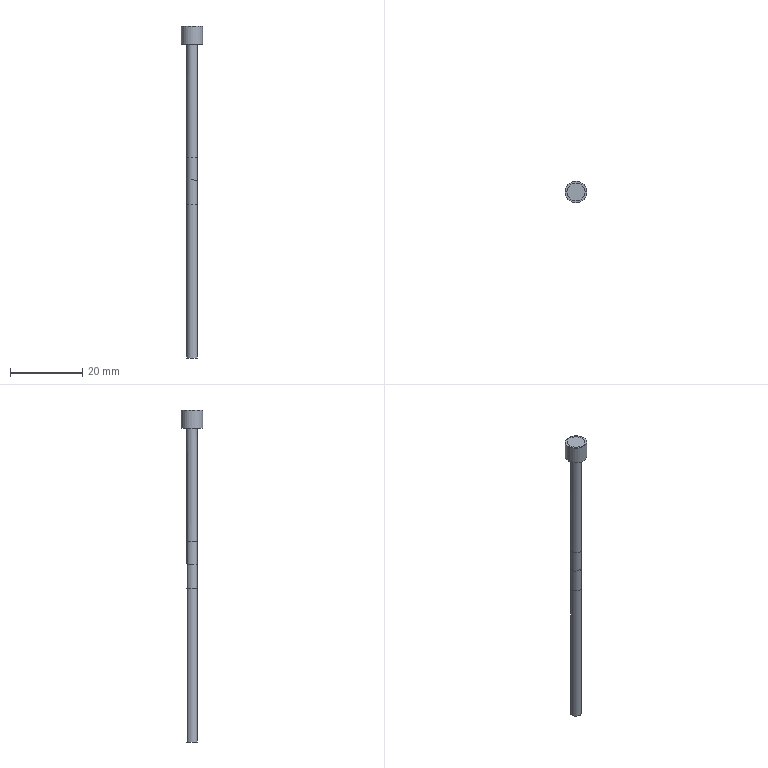Part | NX | features BREP 3 | 3 solids | 38 faces | box 6 x 6 x 92.2 mm | volume 1255 mm3 | cylinder 17 | plane 17 | torus 4 | commonest cylinder face diameters 1 x4 1.1 x4 20 x4 3 x3 5 x1 6 x1
STEP:
#1=CARTESIAN_POINT('',(3.,0.,47.));
#2=VERTEX_POINT('',#1);
#3=CARTESIAN_POINT('',(0.,0.,47.));
#4=DIRECTION('',(0.,0.,-1.));
#5=DIRECTION('',(1.,0.,0.));
#6=AXIS2_PLACEMENT_3D('',#3,#4,#5);
#7=CIRCLE('',#6,3.);
#8=EDGE_CURVE('',#2,#2,#7,.T.);
#9=ORIENTED_EDGE('',*,*,#8,.F.);
#10=EDGE_LOOP('',(#9));
#11=FACE_BOUND('',#10,.T.);
#12=CARTESIAN_POINT('',(3.,0.,52.));
#13=VERTEX_POINT('',#12);
#14=CARTESIAN_POINT('',(0.,0.,52.));
#15=DIRECTION('',(0.,0.,-1.));
#16=DIRECTION('',(1.,0.,0.));
#17=AXIS2_PLACEMENT_3D('',#14,#15,#16);
#18=CIRCLE('',#17,3.);
#19=EDGE_CURVE('',#13,#13,#18,.T.);
#20=ORIENTED_EDGE('',*,*,#19,.T.);
#21=EDGE_LOOP('',(#20));
#22=FACE_BOUND('',#21,.T.);
#23=CARTESIAN_POINT('',(0.,0.,47.));
#24=DIRECTION('',(0.,0.,1.));
#25=DIRECTION('',(-1.,0.,0.));
#26=AXIS2_PLACEMENT_3D('',#23,#24,#25);
#27=CYLINDRICAL_SURFACE('',#26,3.);
#28=ADVANCED_FACE('',(#11,#22),#27,.T.);
#29=CARTESIAN_POINT('',(-1.5,0.,47.));
#30=VERTEX_POINT('',#29);
#31=CARTESIAN_POINT('',(0.,0.,47.));
#32=DIRECTION('',(0.,0.,-1.));
#33=DIRECTION('',(-1.,0.,0.));
#34=AXIS2_PLACEMENT_3D('',#31,#32,#33);
#35=CIRCLE('',#34,1.5);
#36=EDGE_CURVE('',#30,#30,#35,.T.);
#37=ORIENTED_EDGE('',*,*,#36,.F.);
#38=EDGE_LOOP('',(#37));
#39=FACE_BOUND('',#38,.T.);
#40=ORIENTED_EDGE('',*,*,#8,.T.);
#41=EDGE_LOOP('',(#40));
#42=FACE_BOUND('',#41,.T.);
#43=CARTESIAN_POINT('',(0.,0.,47.));
#44=DIRECTION('',(0.,0.,-1.));
#45=DIRECTION('',(1.,0.,0.));
#46=AXIS2_PLACEMENT_3D('',#43,#44,#45);
#47=PLANE('',#46);
#48=ADVANCED_FACE('',(#39,#42),#47,.T.);
#49=ORIENTED_EDGE('',*,*,#19,.F.);
#50=EDGE_LOOP('',(#49));
#51=FACE_BOUND('',#50,.T.);
#52=CARTESIAN_POINT('',(0.,0.,52.));
#53=DIRECTION('',(0.,0.,-1.));
#54=DIRECTION('',(1.,0.,0.));
#55=AXIS2_PLACEMENT_3D('',#52,#53,#54);
#56=PLANE('',#55);
#57=ADVANCED_FACE('',(#51),#56,.F.);
#58=CARTESIAN_POINT('',(-0.25,0.7001,2.4));
#59=VERTEX_POINT('',#58);
#60=CARTESIAN_POINT('',(-0.8001,0.15,2.4));
#61=VERTEX_POINT('',#60);
#62=CARTESIAN_POINT('',(-0.25,0.15,2.4));
#63=DIRECTION('',(0.,0.,1.));
#64=DIRECTION('',(1.,0.,0.));
#65=AXIS2_PLACEMENT_3D('',#62,#63,#64);
#66=CIRCLE('',#65,0.5501);
#67=EDGE_CURVE('',#59,#61,#66,.T.);
#68=ORIENTED_EDGE('',*,*,#67,.T.);
#69=CARTESIAN_POINT('',(-0.8001,-0.15,2.4));
#70=VERTEX_POINT('',#69);
#71=CARTESIAN_POINT('',(-0.8001,0.15,2.4));
#72=DIRECTION('',(0.,-1.,0.));
#73=VECTOR('',#72,1000.);
#74=LINE('',#71,#73);
#75=EDGE_CURVE('',#61,#70,#74,.T.);
#76=ORIENTED_EDGE('',*,*,#75,.T.);
#77=CARTESIAN_POINT('',(-0.25,-0.7001,2.4));
#78=VERTEX_POINT('',#77);
#79=CARTESIAN_POINT('',(-0.25,-0.15,2.4));
#80=DIRECTION('',(0.,0.,1.));
#81=DIRECTION('',(1.,0.,0.));
#82=AXIS2_PLACEMENT_3D('',#79,#80,#81);
#83=CIRCLE('',#82,0.5501);
#84=EDGE_CURVE('',#70,#78,#83,.T.);
#85=ORIENTED_EDGE('',*,*,#84,.T.);
#86=CARTESIAN_POINT('',(0.25,-0.7001,2.4));
#87=VERTEX_POINT('',#86);
#88=CARTESIAN_POINT('',(-0.25,-0.7001,2.4));
#89=DIRECTION('',(1.,0.,0.));
#90=VECTOR('',#89,1000.);
#91=LINE('',#88,#90);
#92=EDGE_CURVE('',#78,#87,#91,.T.);
#93=ORIENTED_EDGE('',*,*,#92,.T.);
#94=CARTESIAN_POINT('',(0.8001,-0.15,2.4));
#95=VERTEX_POINT('',#94);
#96=CARTESIAN_POINT('',(0.25,-0.15,2.4));
#97=DIRECTION('',(0.,0.,1.));
#98=DIRECTION('',(1.,0.,0.));
#99=AXIS2_PLACEMENT_3D('',#96,#97,#98);
#100=CIRCLE('',#99,0.5501);
#101=EDGE_CURVE('',#87,#95,#100,.T.);
#102=ORIENTED_EDGE('',*,*,#101,.T.);
#103=CARTESIAN_POINT('',(0.8001,0.15,2.4));
#104=VERTEX_POINT('',#103);
#105=CARTESIAN_POINT('',(0.8001,-0.15,2.4));
#106=DIRECTION('',(0.,1.,0.));
#107=VECTOR('',#106,1000.);
#108=LINE('',#105,#107);
#109=EDGE_CURVE('',#95,#104,#108,.T.);
#110=ORIENTED_EDGE('',*,*,#109,.T.);
#111=CARTESIAN_POINT('',(0.25,0.7001,2.4));
#112=VERTEX_POINT('',#111);
#113=CARTESIAN_POINT('',(0.25,0.15,2.4));
#114=DIRECTION('',(0.,0.,1.));
#115=DIRECTION('',(1.,0.,0.));
#116=AXIS2_PLACEMENT_3D('',#113,#114,#115);
#117=CIRCLE('',#116,0.5501);
#118=EDGE_CURVE('',#104,#112,#117,.T.);
#119=ORIENTED_EDGE('',*,*,#118,.T.);
#120=CARTESIAN_POINT('',(0.25,0.7001,2.4));
#121=DIRECTION('',(-1.,0.,0.));
#122=VECTOR('',#121,1000.);
#123=LINE('',#120,#122);
#124=EDGE_CURVE('',#112,#59,#123,.T.);
#125=ORIENTED_EDGE('',*,*,#124,.T.);
#126=EDGE_LOOP('',(#68,#76,#85,#93,#102,#110,#119,#125));
#127=FACE_BOUND('',#126,.T.);
#128=CARTESIAN_POINT('',(-1.5,0.,2.4));
#129=VERTEX_POINT('',#128);
#130=CARTESIAN_POINT('',(0.,0.,2.4));
#131=DIRECTION('',(0.,0.,-1.));
#132=DIRECTION('',(-1.,0.,0.));
#133=AXIS2_PLACEMENT_3D('',#130,#131,#132);
#134=CIRCLE('',#133,1.5);
#135=EDGE_CURVE('',#129,#129,#134,.T.);
#136=ORIENTED_EDGE('',*,*,#135,.T.);
#137=EDGE_LOOP('',(#136));
#138=FACE_BOUND('',#137,.T.);
#139=CARTESIAN_POINT('',(0.,0.,2.4));
#140=DIRECTION('',(0.,0.,-1.));
#141=DIRECTION('',(1.,0.,0.));
#142=AXIS2_PLACEMENT_3D('',#139,#140,#141);
#143=PLANE('',#142);
#144=ADVANCED_FACE('',(#127,#138),#143,.T.);
#145=ORIENTED_EDGE('',*,*,#135,.F.);
#146=EDGE_LOOP('',(#145));
#147=FACE_BOUND('',#146,.T.);
#148=ORIENTED_EDGE('',*,*,#36,.T.);
#149=EDGE_LOOP('',(#148));
#150=FACE_BOUND('',#149,.T.);
#151=CARTESIAN_POINT('',(0.,0.,47.));
#152=DIRECTION('',(0.,0.,-1.));
#153=DIRECTION('',(1.,0.,0.));
#154=AXIS2_PLACEMENT_3D('',#151,#152,#153);
#155=CYLINDRICAL_SURFACE('',#154,1.5);
#156=ADVANCED_FACE('',(#147,#150),#155,.T.);
#157=CARTESIAN_POINT('',(-0.25,-0.7001,-3.6));
#158=VERTEX_POINT('',#157);
#159=CARTESIAN_POINT('',(-0.25,-0.7001,0.));
#160=DIRECTION('',(0.,0.,-1.));
#161=VECTOR('',#160,1000.);
#162=LINE('',#159,#161);
#163=EDGE_CURVE('',#78,#158,#162,.T.);
#164=ORIENTED_EDGE('',*,*,#163,.T.);
#165=CARTESIAN_POINT('',(0.25,-0.7001,-3.6));
#166=VERTEX_POINT('',#165);
#167=CARTESIAN_POINT('',(-0.25,-0.7001,-3.6));
#168=DIRECTION('',(1.,0.,0.));
#169=VECTOR('',#168,1000.);
#170=LINE('',#167,#169);
#171=EDGE_CURVE('',#158,#166,#170,.T.);
#172=ORIENTED_EDGE('',*,*,#171,.T.);
#173=CARTESIAN_POINT('',(0.25,-0.7001,0.));
#174=DIRECTION('',(0.,0.,-1.));
#175=VECTOR('',#174,1000.);
#176=LINE('',#173,#175);
#177=EDGE_CURVE('',#87,#166,#176,.T.);
#178=ORIENTED_EDGE('',*,*,#177,.F.);
#179=ORIENTED_EDGE('',*,*,#92,.F.);
#180=EDGE_LOOP('',(#164,#172,#178,#179));
#181=FACE_BOUND('',#180,.T.);
#182=CARTESIAN_POINT('',(-0.25,-0.7001,0.));
#183=DIRECTION('',(0.,-1.,0.));
#184=DIRECTION('',(-1.,0.,0.));
#185=AXIS2_PLACEMENT_3D('',#182,#183,#184);
#186=PLANE('',#185);
#187=ADVANCED_FACE('',(#181),#186,.T.);
#188=ORIENTED_EDGE('',*,*,#177,.T.);
#189=CARTESIAN_POINT('',(0.8001,-0.15,-3.6));
#190=VERTEX_POINT('',#189);
#191=CARTESIAN_POINT('',(0.25,-0.15,-3.6));
#192=DIRECTION('',(0.,0.,1.));
#193=DIRECTION('',(1.,0.,0.));
#194=AXIS2_PLACEMENT_3D('',#191,#192,#193);
#195=CIRCLE('',#194,0.5501);
#196=EDGE_CURVE('',#166,#190,#195,.T.);
#197=ORIENTED_EDGE('',*,*,#196,.T.);
#198=CARTESIAN_POINT('',(0.8001,-0.15,0.));
#199=DIRECTION('',(0.,0.,-1.));
#200=VECTOR('',#199,1000.);
#201=LINE('',#198,#200);
#202=EDGE_CURVE('',#95,#190,#201,.T.);
#203=ORIENTED_EDGE('',*,*,#202,.F.);
#204=ORIENTED_EDGE('',*,*,#101,.F.);
#205=EDGE_LOOP('',(#188,#197,#203,#204));
#206=FACE_BOUND('',#205,.T.);
#207=CARTESIAN_POINT('',(0.25,-0.15,0.));
#208=DIRECTION('',(0.,0.,1.));
#209=DIRECTION('',(-1.,0.,0.));
#210=AXIS2_PLACEMENT_3D('',#207,#208,#209);
#211=CYLINDRICAL_SURFACE('',#210,0.5501);
#212=ADVANCED_FACE('',(#206),#211,.T.);
#213=ORIENTED_EDGE('',*,*,#202,.T.);
#214=CARTESIAN_POINT('',(0.8001,0.15,-3.6));
#215=VERTEX_POINT('',#214);
#216=CARTESIAN_POINT('',(0.8001,-0.15,-3.6));
#217=DIRECTION('',(0.,1.,0.));
#218=VECTOR('',#217,1000.);
#219=LINE('',#216,#218);
#220=EDGE_CURVE('',#190,#215,#219,.T.);
#221=ORIENTED_EDGE('',*,*,#220,.T.);
#222=CARTESIAN_POINT('',(0.8001,0.15,0.));
#223=DIRECTION('',(0.,0.,-1.));
#224=VECTOR('',#223,1000.);
#225=LINE('',#222,#224);
#226=EDGE_CURVE('',#104,#215,#225,.T.);
#227=ORIENTED_EDGE('',*,*,#226,.F.);
#228=ORIENTED_EDGE('',*,*,#109,.F.);
#229=EDGE_LOOP('',(#213,#221,#227,#228));
#230=FACE_BOUND('',#229,.T.);
#231=CARTESIAN_POINT('',(0.8001,-0.15,0.));
#232=DIRECTION('',(1.,0.,0.));
#233=DIRECTION('',(0.,-1.,0.));
#234=AXIS2_PLACEMENT_3D('',#231,#232,#233);
#235=PLANE('',#234);
#236=ADVANCED_FACE('',(#230),#235,.T.);
#237=ORIENTED_EDGE('',*,*,#226,.T.);
#238=CARTESIAN_POINT('',(0.25,0.7001,-3.6));
#239=VERTEX_POINT('',#238);
#240=CARTESIAN_POINT('',(0.25,0.15,-3.6));
#241=DIRECTION('',(0.,0.,1.));
#242=DIRECTION('',(1.,0.,0.));
#243=AXIS2_PLACEMENT_3D('',#240,#241,#242);
#244=CIRCLE('',#243,0.5501);
#245=EDGE_CURVE('',#215,#239,#244,.T.);
#246=ORIENTED_EDGE('',*,*,#245,.T.);
#247=CARTESIAN_POINT('',(0.25,0.7001,0.));
#248=DIRECTION('',(0.,0.,-1.));
#249=VECTOR('',#248,1000.);
#250=LINE('',#247,#249);
#251=EDGE_CURVE('',#112,#239,#250,.T.);
#252=ORIENTED_EDGE('',*,*,#251,.F.);
#253=ORIENTED_EDGE('',*,*,#118,.F.);
#254=EDGE_LOOP('',(#237,#246,#252,#253));
#255=FACE_BOUND('',#254,.T.);
#256=CARTESIAN_POINT('',(0.25,0.15,0.));
#257=DIRECTION('',(0.,0.,1.));
#258=DIRECTION('',(-1.,0.,0.));
#259=AXIS2_PLACEMENT_3D('',#256,#257,#258);
#260=CYLINDRICAL_SURFACE('',#259,0.5501);
#261=ADVANCED_FACE('',(#255),#260,.T.);
#262=ORIENTED_EDGE('',*,*,#251,.T.);
#263=CARTESIAN_POINT('',(-0.25,0.7001,-3.6));
#264=VERTEX_POINT('',#263);
#265=CARTESIAN_POINT('',(0.25,0.7001,-3.6));
#266=DIRECTION('',(-1.,0.,0.));
#267=VECTOR('',#266,1000.);
#268=LINE('',#265,#267);
#269=EDGE_CURVE('',#239,#264,#268,.T.);
#270=ORIENTED_EDGE('',*,*,#269,.T.);
#271=CARTESIAN_POINT('',(-0.25,0.7001,0.));
#272=DIRECTION('',(0.,0.,-1.));
#273=VECTOR('',#272,1000.);
#274=LINE('',#271,#273);
#275=EDGE_CURVE('',#59,#264,#274,.T.);
#276=ORIENTED_EDGE('',*,*,#275,.F.);
#277=ORIENTED_EDGE('',*,*,#124,.F.);
#278=EDGE_LOOP('',(#262,#270,#276,#277));
#279=FACE_BOUND('',#278,.T.);
#280=CARTESIAN_POINT('',(0.25,0.7001,0.));
#281=DIRECTION('',(0.,1.,0.));
#282=DIRECTION('',(1.,0.,0.));
#283=AXIS2_PLACEMENT_3D('',#280,#281,#282);
#284=PLANE('',#283);
#285=ADVANCED_FACE('',(#279),#284,.T.);
#286=ORIENTED_EDGE('',*,*,#275,.T.);
#287=CARTESIAN_POINT('',(-0.8001,0.15,-3.6));
#288=VERTEX_POINT('',#287);
#289=CARTESIAN_POINT('',(-0.25,0.15,-3.6));
#290=DIRECTION('',(0.,0.,1.));
#291=DIRECTION('',(1.,0.,0.));
#292=AXIS2_PLACEMENT_3D('',#289,#290,#291);
#293=CIRCLE('',#292,0.5501);
#294=EDGE_CURVE('',#264,#288,#293,.T.);
#295=ORIENTED_EDGE('',*,*,#294,.T.);
#296=CARTESIAN_POINT('',(-0.8001,0.15,0.));
#297=DIRECTION('',(0.,0.,-1.));
#298=VECTOR('',#297,1000.);
#299=LINE('',#296,#298);
#300=EDGE_CURVE('',#61,#288,#299,.T.);
#301=ORIENTED_EDGE('',*,*,#300,.F.);
#302=ORIENTED_EDGE('',*,*,#67,.F.);
#303=EDGE_LOOP('',(#286,#295,#301,#302));
#304=FACE_BOUND('',#303,.T.);
#305=CARTESIAN_POINT('',(-0.25,0.15,0.));
#306=DIRECTION('',(0.,0.,1.));
#307=DIRECTION('',(-1.,0.,0.));
#308=AXIS2_PLACEMENT_3D('',#305,#306,#307);
#309=CYLINDRICAL_SURFACE('',#308,0.5501);
#310=ADVANCED_FACE('',(#304),#309,.T.);
#311=ORIENTED_EDGE('',*,*,#300,.T.);
#312=CARTESIAN_POINT('',(-0.8001,-0.15,-3.6));
#313=VERTEX_POINT('',#312);
#314=CARTESIAN_POINT('',(-0.8001,0.15,-3.6));
#315=DIRECTION('',(0.,-1.,0.));
#316=VECTOR('',#315,1000.);
#317=LINE('',#314,#316);
#318=EDGE_CURVE('',#288,#313,#317,.T.);
#319=ORIENTED_EDGE('',*,*,#318,.T.);
#320=CARTESIAN_POINT('',(-0.8001,-0.15,0.));
#321=DIRECTION('',(0.,0.,-1.));
#322=VECTOR('',#321,1000.);
#323=LINE('',#320,#322);
#324=EDGE_CURVE('',#70,#313,#323,.T.);
#325=ORIENTED_EDGE('',*,*,#324,.F.);
#326=ORIENTED_EDGE('',*,*,#75,.F.);
#327=EDGE_LOOP('',(#311,#319,#325,#326));
#328=FACE_BOUND('',#327,.T.);
#329=CARTESIAN_POINT('',(-0.8001,0.15,0.));
#330=DIRECTION('',(-1.,0.,0.));
#331=DIRECTION('',(0.,1.,0.));
#332=AXIS2_PLACEMENT_3D('',#329,#330,#331);
#333=PLANE('',#332);
#334=ADVANCED_FACE('',(#328),#333,.T.);
#335=ORIENTED_EDGE('',*,*,#84,.F.);
#336=ORIENTED_EDGE('',*,*,#324,.T.);
#337=CARTESIAN_POINT('',(-0.25,-0.15,-3.6));
#338=DIRECTION('',(0.,0.,1.));
#339=DIRECTION('',(1.,0.,0.));
#340=AXIS2_PLACEMENT_3D('',#337,#338,#339);
#341=CIRCLE('',#340,0.5501);
#342=EDGE_CURVE('',#313,#158,#341,.T.);
#343=ORIENTED_EDGE('',*,*,#342,.T.);
#344=ORIENTED_EDGE('',*,*,#163,.F.);
#345=EDGE_LOOP('',(#335,#336,#343,#344));
#346=FACE_BOUND('',#345,.T.);
#347=CARTESIAN_POINT('',(-0.25,-0.15,0.));
#348=DIRECTION('',(0.,0.,1.));
#349=DIRECTION('',(-1.,0.,0.));
#350=AXIS2_PLACEMENT_3D('',#347,#348,#349);
#351=CYLINDRICAL_SURFACE('',#350,0.5501);
#352=ADVANCED_FACE('',(#346),#351,.T.);
#353=ORIENTED_EDGE('',*,*,#318,.F.);
#354=ORIENTED_EDGE('',*,*,#294,.F.);
#355=ORIENTED_EDGE('',*,*,#269,.F.);
#356=ORIENTED_EDGE('',*,*,#245,.F.);
#357=ORIENTED_EDGE('',*,*,#220,.F.);
#358=ORIENTED_EDGE('',*,*,#196,.F.);
#359=ORIENTED_EDGE('',*,*,#171,.F.);
#360=ORIENTED_EDGE('',*,*,#342,.F.);
#361=EDGE_LOOP('',(#353,#354,#355,#356,#357,#358,#359,#360));
#362=FACE_BOUND('',#361,.T.);
#363=CARTESIAN_POINT('',(8.223,0.1277,-3.6));
#364=DIRECTION('',(0.,0.,1.));
#365=DIRECTION('',(-1.,0.,0.));
#366=AXIS2_PLACEMENT_3D('',#363,#364,#365);
#367=PLANE('',#366);
#368=ADVANCED_FACE('',(#362),#367,.F.);
#369=CLOSED_SHELL('',(#28,#48,#57,#144,#156,#187,#212,#236,#261,#285,#310,#334,#352,#368));
#370=MANIFOLD_SOLID_BREP('',#369);
#371=CARTESIAN_POINT('',(2.5,0.,47.));
#372=VERTEX_POINT('',#371);
#373=CARTESIAN_POINT('',(0.,0.,47.));
#374=DIRECTION('',(0.,0.,-1.));
#375=DIRECTION('',(1.,0.,0.));
#376=AXIS2_PLACEMENT_3D('',#373,#374,#375);
#377=CIRCLE('',#376,2.5);
#378=EDGE_CURVE('',#372,#372,#377,.T.);
#379=ORIENTED_EDGE('',*,*,#378,.F.);
#380=EDGE_LOOP('',(#379));
#381=FACE_BOUND('',#380,.T.);
#382=CARTESIAN_POINT('',(2.5,0.,52.));
#383=VERTEX_POINT('',#382);
#384=CARTESIAN_POINT('',(0.,0.,52.));
#385=DIRECTION('',(0.,0.,-1.));
#386=DIRECTION('',(1.,0.,0.));
#387=AXIS2_PLACEMENT_3D('',#384,#385,#386);
#388=CIRCLE('',#387,2.5);
#389=EDGE_CURVE('',#383,#383,#388,.T.);
#390=ORIENTED_EDGE('',*,*,#389,.T.);
#391=EDGE_LOOP('',(#390));
#392=FACE_BOUND('',#391,.T.);
#393=CARTESIAN_POINT('',(0.,0.,47.));
#394=DIRECTION('',(0.,0.,1.));
#395=DIRECTION('',(-1.,0.,0.));
#396=AXIS2_PLACEMENT_3D('',#393,#394,#395);
#397=CYLINDRICAL_SURFACE('',#396,2.5);
#398=ADVANCED_FACE('',(#381,#392),#397,.T.);
#399=CARTESIAN_POINT('',(-1.5,0.,47.));
#400=VERTEX_POINT('',#399);
#401=CARTESIAN_POINT('',(0.,0.,47.));
#402=DIRECTION('',(0.,0.,-1.));
#403=DIRECTION('',(-1.,0.,0.));
#404=AXIS2_PLACEMENT_3D('',#401,#402,#403);
#405=CIRCLE('',#404,1.5);
#406=EDGE_CURVE('',#400,#400,#405,.T.);
#407=ORIENTED_EDGE('',*,*,#406,.F.);
#408=EDGE_LOOP('',(#407));
#409=FACE_BOUND('',#408,.T.);
#410=ORIENTED_EDGE('',*,*,#378,.T.);
#411=EDGE_LOOP('',(#410));
#412=FACE_BOUND('',#411,.T.);
#413=CARTESIAN_POINT('',(0.,0.,47.));
#414=DIRECTION('',(0.,0.,-1.));
#415=DIRECTION('',(1.,0.,0.));
#416=AXIS2_PLACEMENT_3D('',#413,#414,#415);
#417=PLANE('',#416);
#418=ADVANCED_FACE('',(#409,#412),#417,.T.);
#419=ORIENTED_EDGE('',*,*,#389,.F.);
#420=EDGE_LOOP('',(#419));
#421=FACE_BOUND('',#420,.T.);
#422=CARTESIAN_POINT('',(0.,0.,52.));
#423=DIRECTION('',(0.,0.,-1.));
#424=DIRECTION('',(1.,0.,0.));
#425=AXIS2_PLACEMENT_3D('',#422,#423,#424);
#426=PLANE('',#425);
#427=ADVANCED_FACE('',(#421),#426,.F.);
#428=ORIENTED_EDGE('',*,*,#406,.T.);
#429=EDGE_LOOP('',(#428));
#430=FACE_BOUND('',#429,.T.);
#431=CARTESIAN_POINT('',(-1.492,-0.15,9.181));
#432=VERTEX_POINT('',#431);
#433=CARTESIAN_POINT('',(-1.492,0.15,9.181));
#434=VERTEX_POINT('',#433);
#435=CARTESIAN_POINT('',(-1.492,-0.15,9.181));
#436=CARTESIAN_POINT('',(-1.502,-0.05157,9.205));
#437=CARTESIAN_POINT('',(-1.502,0.05153,9.205));
#438=CARTESIAN_POINT('',(-1.492,0.15,9.181));
#439=B_SPLINE_CURVE_WITH_KNOTS('',3,(#435,#436,#437,#438),.UNSPECIFIED.,.F.,.F.,(4,4),(0.,0.0003013),.UNSPECIFIED.);
#440=EDGE_CURVE('',#432,#434,#439,.T.);
#441=ORIENTED_EDGE('',*,*,#440,.F.);
#442=CARTESIAN_POINT('',(-0.25,-1.479,9.386));
#443=VERTEX_POINT('',#442);
#444=CARTESIAN_POINT('',(-0.25,-1.479,9.386));
#445=CARTESIAN_POINT('',(-0.8693,-1.374,9.146));
#446=CARTESIAN_POINT('',(-1.427,-0.8014,9.021));
#447=CARTESIAN_POINT('',(-1.492,-0.15,9.181));
#448=B_SPLINE_CURVE_WITH_KNOTS('',3,(#444,#445,#446,#447),.UNSPECIFIED.,.F.,.F.,(4,4),(0.,0.001996),.UNSPECIFIED.);
#449=EDGE_CURVE('',#443,#432,#448,.T.);
#450=ORIENTED_EDGE('',*,*,#449,.F.);
#451=CARTESIAN_POINT('',(0.25,-1.479,9.386));
#452=VERTEX_POINT('',#451);
#453=CARTESIAN_POINT('',(0.25,-1.479,9.386));
#454=CARTESIAN_POINT('',(0.09098,-1.506,9.448));
#455=CARTESIAN_POINT('',(-0.09088,-1.506,9.448));
#456=CARTESIAN_POINT('',(-0.25,-1.479,9.386));
#457=B_SPLINE_CURVE_WITH_KNOTS('',3,(#453,#454,#455,#456),.UNSPECIFIED.,.F.,.F.,(4,4),(0.,0.0005114),.UNSPECIFIED.);
#458=EDGE_CURVE('',#452,#443,#457,.T.);
#459=ORIENTED_EDGE('',*,*,#458,.F.);
#460=CARTESIAN_POINT('',(1.492,-0.15,9.181));
#461=VERTEX_POINT('',#460);
#462=CARTESIAN_POINT('',(1.492,-0.15,9.181));
#463=CARTESIAN_POINT('',(1.427,-0.8,9.021));
#464=CARTESIAN_POINT('',(0.8687,-1.374,9.146));
#465=CARTESIAN_POINT('',(0.25,-1.479,9.386));
#466=B_SPLINE_CURVE_WITH_KNOTS('',3,(#462,#463,#464,#465),.UNSPECIFIED.,.F.,.F.,(4,4),(0.,0.00199),.UNSPECIFIED.);
#467=EDGE_CURVE('',#461,#452,#466,.T.);
#468=ORIENTED_EDGE('',*,*,#467,.F.);
#469=CARTESIAN_POINT('',(1.492,0.15,9.181));
#470=VERTEX_POINT('',#469);
#471=CARTESIAN_POINT('',(1.492,0.15,9.181));
#472=CARTESIAN_POINT('',(1.502,0.05157,9.205));
#473=CARTESIAN_POINT('',(1.502,-0.05153,9.205));
#474=CARTESIAN_POINT('',(1.492,-0.15,9.181));
#475=B_SPLINE_CURVE_WITH_KNOTS('',3,(#471,#472,#473,#474),.UNSPECIFIED.,.F.,.F.,(4,4),(0.,0.0003013),.UNSPECIFIED.);
#476=EDGE_CURVE('',#470,#461,#475,.T.);
#477=ORIENTED_EDGE('',*,*,#476,.F.);
#478=CARTESIAN_POINT('',(0.25,1.479,9.386));
#479=VERTEX_POINT('',#478);
#480=CARTESIAN_POINT('',(0.25,1.479,9.386));
#481=CARTESIAN_POINT('',(0.8693,1.374,9.146));
#482=CARTESIAN_POINT('',(1.427,0.8014,9.021));
#483=CARTESIAN_POINT('',(1.492,0.15,9.181));
#484=B_SPLINE_CURVE_WITH_KNOTS('',3,(#480,#481,#482,#483),.UNSPECIFIED.,.F.,.F.,(4,4),(0.,0.001996),.UNSPECIFIED.);
#485=EDGE_CURVE('',#479,#470,#484,.T.);
#486=ORIENTED_EDGE('',*,*,#485,.F.);
#487=CARTESIAN_POINT('',(-0.25,1.479,9.386));
#488=VERTEX_POINT('',#487);
#489=CARTESIAN_POINT('',(-0.25,1.479,9.386));
#490=CARTESIAN_POINT('',(-0.09098,1.506,9.448));
#491=CARTESIAN_POINT('',(0.09088,1.506,9.448));
#492=CARTESIAN_POINT('',(0.25,1.479,9.386));
#493=B_SPLINE_CURVE_WITH_KNOTS('',3,(#489,#490,#491,#492),.UNSPECIFIED.,.F.,.F.,(4,4),(0.,0.0005114),.UNSPECIFIED.);
#494=EDGE_CURVE('',#488,#479,#493,.T.);
#495=ORIENTED_EDGE('',*,*,#494,.F.);
#496=CARTESIAN_POINT('',(-1.492,0.15,9.181));
#497=CARTESIAN_POINT('',(-1.427,0.8,9.021));
#498=CARTESIAN_POINT('',(-0.8687,1.374,9.146));
#499=CARTESIAN_POINT('',(-0.25,1.479,9.386));
#500=B_SPLINE_CURVE_WITH_KNOTS('',3,(#496,#497,#498,#499),.UNSPECIFIED.,.F.,.F.,(4,4),(0.,0.00199),.UNSPECIFIED.);
#501=EDGE_CURVE('',#434,#488,#500,.T.);
#502=ORIENTED_EDGE('',*,*,#501,.F.);
#503=EDGE_LOOP('',(#441,#450,#459,#468,#477,#486,#495,#502));
#504=FACE_BOUND('',#503,.T.);
#505=CARTESIAN_POINT('',(0.,0.,47.));
#506=DIRECTION('',(0.,0.,-1.));
#507=DIRECTION('',(1.,0.,0.));
#508=AXIS2_PLACEMENT_3D('',#505,#506,#507);
#509=CYLINDRICAL_SURFACE('',#508,1.5);
#510=ADVANCED_FACE('',(#430,#504),#509,.T.);
#511=CARTESIAN_POINT('',(-0.7501,-0.15,5.4));
#512=VERTEX_POINT('',#511);
#513=CARTESIAN_POINT('',(-10.75,-0.15,5.4));
#514=DIRECTION('',(0.,-1.,0.));
#515=DIRECTION('',(1.,0.,0.));
#516=AXIS2_PLACEMENT_3D('',#513,#514,#515);
#517=CIRCLE('',#516,10.);
#518=EDGE_CURVE('',#512,#432,#517,.T.);
#519=ORIENTED_EDGE('',*,*,#518,.T.);
#520=ORIENTED_EDGE('',*,*,#440,.T.);
#521=CARTESIAN_POINT('',(-0.7501,0.15,5.4));
#522=VERTEX_POINT('',#521);
#523=CARTESIAN_POINT('',(-10.75,0.15,5.4));
#524=DIRECTION('',(0.,-1.,0.));
#525=DIRECTION('',(0.,0.,-1.));
#526=AXIS2_PLACEMENT_3D('',#523,#524,#525);
#527=CIRCLE('',#526,10.);
#528=EDGE_CURVE('',#522,#434,#527,.T.);
#529=ORIENTED_EDGE('',*,*,#528,.F.);
#530=CARTESIAN_POINT('',(-0.7501,0.15,5.4));
#531=DIRECTION('',(0.,1.,0.));
#532=VECTOR('',#531,1000.);
#533=LINE('',#530,#532);
#534=EDGE_CURVE('',#512,#522,#533,.T.);
#535=ORIENTED_EDGE('',*,*,#534,.F.);
#536=EDGE_LOOP('',(#519,#520,#529,#535));
#537=FACE_BOUND('',#536,.T.);
#538=CARTESIAN_POINT('',(-10.75,0.15,5.4));
#539=DIRECTION('',(0.,-1.,0.));
#540=DIRECTION('',(0.,0.,1.));
#541=AXIS2_PLACEMENT_3D('',#538,#539,#540);
#542=CYLINDRICAL_SURFACE('',#541,10.);
#543=ADVANCED_FACE('',(#537),#542,.F.);
#544=CARTESIAN_POINT('',(-0.25,-0.6501,5.4));
#545=VERTEX_POINT('',#544);
#546=CARTESIAN_POINT('',(-0.25,-10.65,5.4));
#547=DIRECTION('',(1.,0.,0.));
#548=DIRECTION('',(0.,1.,0.));
#549=AXIS2_PLACEMENT_3D('',#546,#547,#548);
#550=CIRCLE('',#549,10.);
#551=EDGE_CURVE('',#545,#443,#550,.T.);
#552=ORIENTED_EDGE('',*,*,#551,.T.);
#553=ORIENTED_EDGE('',*,*,#449,.T.);
#554=ORIENTED_EDGE('',*,*,#518,.F.);
#555=CARTESIAN_POINT('',(-0.25,-0.15,5.4));
#556=DIRECTION('',(0.,0.,-1.));
#557=DIRECTION('',(-1.,0.,0.));
#558=AXIS2_PLACEMENT_3D('',#555,#556,#557);
#559=CIRCLE('',#558,0.5001);
#560=EDGE_CURVE('',#545,#512,#559,.T.);
#561=ORIENTED_EDGE('',*,*,#560,.F.);
#562=EDGE_LOOP('',(#552,#553,#554,#561));
#563=FACE_BOUND('',#562,.T.);
#564=CARTESIAN_POINT('',(-0.25,-0.15,5.4));
#565=DIRECTION('',(0.,0.,-1.));
#566=DIRECTION('',(1.,0.,0.));
#567=AXIS2_PLACEMENT_3D('',#564,#565,#566);
#568=TOROIDAL_SURFACE('',#567,10.5,10.);
#569=ADVANCED_FACE('',(#563),#568,.F.);
#570=CARTESIAN_POINT('',(0.25,-0.6501,5.4));
#571=VERTEX_POINT('',#570);
#572=CARTESIAN_POINT('',(0.25,-10.65,5.4));
#573=DIRECTION('',(1.,0.,0.));
#574=DIRECTION('',(0.,1.,0.));
#575=AXIS2_PLACEMENT_3D('',#572,#573,#574);
#576=CIRCLE('',#575,10.);
#577=EDGE_CURVE('',#571,#452,#576,.T.);
#578=ORIENTED_EDGE('',*,*,#577,.T.);
#579=ORIENTED_EDGE('',*,*,#458,.T.);
#580=ORIENTED_EDGE('',*,*,#551,.F.);
#581=CARTESIAN_POINT('',(-0.25,-0.6501,5.4));
#582=DIRECTION('',(-1.,0.,0.));
#583=VECTOR('',#582,1000.);
#584=LINE('',#581,#583);
#585=EDGE_CURVE('',#571,#545,#584,.T.);
#586=ORIENTED_EDGE('',*,*,#585,.F.);
#587=EDGE_LOOP('',(#578,#579,#580,#586));
#588=FACE_BOUND('',#587,.T.);
#589=CARTESIAN_POINT('',(-0.25,-10.65,5.4));
#590=DIRECTION('',(1.,0.,0.));
#591=DIRECTION('',(0.,-1.,0.));
#592=AXIS2_PLACEMENT_3D('',#589,#590,#591);
#593=CYLINDRICAL_SURFACE('',#592,10.);
#594=ADVANCED_FACE('',(#588),#593,.F.);
#595=CARTESIAN_POINT('',(0.7501,-0.15,5.4));
#596=VERTEX_POINT('',#595);
#597=CARTESIAN_POINT('',(10.75,-0.15,5.4));
#598=DIRECTION('',(0.,1.,0.));
#599=DIRECTION('',(0.,0.,1.));
#600=AXIS2_PLACEMENT_3D('',#597,#598,#599);
#601=CIRCLE('',#600,10.);
#602=EDGE_CURVE('',#596,#461,#601,.T.);
#603=ORIENTED_EDGE('',*,*,#602,.T.);
#604=ORIENTED_EDGE('',*,*,#467,.T.);
#605=ORIENTED_EDGE('',*,*,#577,.F.);
#606=CARTESIAN_POINT('',(0.25,-0.15,5.4));
#607=DIRECTION('',(0.,0.,-1.));
#608=DIRECTION('',(-1.,0.,0.));
#609=AXIS2_PLACEMENT_3D('',#606,#607,#608);
#610=CIRCLE('',#609,0.5001);
#611=EDGE_CURVE('',#596,#571,#610,.T.);
#612=ORIENTED_EDGE('',*,*,#611,.F.);
#613=EDGE_LOOP('',(#603,#604,#605,#612));
#614=FACE_BOUND('',#613,.T.);
#615=CARTESIAN_POINT('',(0.25,-0.15,5.4));
#616=DIRECTION('',(0.,0.,-1.));
#617=DIRECTION('',(1.,0.,0.));
#618=AXIS2_PLACEMENT_3D('',#615,#616,#617);
#619=TOROIDAL_SURFACE('',#618,10.5,10.);
#620=ADVANCED_FACE('',(#614),#619,.F.);
#621=CARTESIAN_POINT('',(0.7501,0.15,5.4));
#622=VERTEX_POINT('',#621);
#623=CARTESIAN_POINT('',(10.75,0.15,5.4));
#624=DIRECTION('',(0.,1.,0.));
#625=DIRECTION('',(0.,0.,1.));
#626=AXIS2_PLACEMENT_3D('',#623,#624,#625);
#627=CIRCLE('',#626,10.);
#628=EDGE_CURVE('',#622,#470,#627,.T.);
#629=ORIENTED_EDGE('',*,*,#628,.T.);
#630=ORIENTED_EDGE('',*,*,#476,.T.);
#631=ORIENTED_EDGE('',*,*,#602,.F.);
#632=CARTESIAN_POINT('',(0.7501,-0.15,5.4));
#633=DIRECTION('',(0.,-1.,0.));
#634=VECTOR('',#633,1000.);
#635=LINE('',#632,#634);
#636=EDGE_CURVE('',#622,#596,#635,.T.);
#637=ORIENTED_EDGE('',*,*,#636,.F.);
#638=EDGE_LOOP('',(#629,#630,#631,#637));
#639=FACE_BOUND('',#638,.T.);
#640=CARTESIAN_POINT('',(10.75,-0.15,5.4));
#641=DIRECTION('',(0.,1.,0.));
#642=DIRECTION('',(0.,0.,-1.));
#643=AXIS2_PLACEMENT_3D('',#640,#641,#642);
#644=CYLINDRICAL_SURFACE('',#643,10.);
#645=ADVANCED_FACE('',(#639),#644,.F.);
#646=CARTESIAN_POINT('',(0.25,0.6501,5.4));
#647=VERTEX_POINT('',#646);
#648=CARTESIAN_POINT('',(0.25,10.65,5.4));
#649=DIRECTION('',(-1.,0.,0.));
#650=DIRECTION('',(0.,-1.,0.));
#651=AXIS2_PLACEMENT_3D('',#648,#649,#650);
#652=CIRCLE('',#651,10.);
#653=EDGE_CURVE('',#647,#479,#652,.T.);
#654=ORIENTED_EDGE('',*,*,#653,.T.);
#655=ORIENTED_EDGE('',*,*,#485,.T.);
#656=ORIENTED_EDGE('',*,*,#628,.F.);
#657=CARTESIAN_POINT('',(0.25,0.15,5.4));
#658=DIRECTION('',(0.,0.,-1.));
#659=DIRECTION('',(-1.,0.,0.));
#660=AXIS2_PLACEMENT_3D('',#657,#658,#659);
#661=CIRCLE('',#660,0.5001);
#662=EDGE_CURVE('',#647,#622,#661,.T.);
#663=ORIENTED_EDGE('',*,*,#662,.F.);
#664=EDGE_LOOP('',(#654,#655,#656,#663));
#665=FACE_BOUND('',#664,.T.);
#666=CARTESIAN_POINT('',(0.25,0.15,5.4));
#667=DIRECTION('',(0.,0.,-1.));
#668=DIRECTION('',(1.,0.,0.));
#669=AXIS2_PLACEMENT_3D('',#666,#667,#668);
#670=TOROIDAL_SURFACE('',#669,10.5,10.);
#671=ADVANCED_FACE('',(#665),#670,.F.);
#672=CARTESIAN_POINT('',(-0.25,0.6501,5.4));
#673=VERTEX_POINT('',#672);
#674=CARTESIAN_POINT('',(-0.25,10.65,5.4));
#675=DIRECTION('',(-1.,0.,0.));
#676=DIRECTION('',(0.,-1.,0.));
#677=AXIS2_PLACEMENT_3D('',#674,#675,#676);
#678=CIRCLE('',#677,10.);
#679=EDGE_CURVE('',#673,#488,#678,.T.);
#680=ORIENTED_EDGE('',*,*,#679,.T.);
#681=ORIENTED_EDGE('',*,*,#494,.T.);
#682=ORIENTED_EDGE('',*,*,#653,.F.);
#683=CARTESIAN_POINT('',(0.25,0.6501,5.4));
#684=DIRECTION('',(1.,0.,0.));
#685=VECTOR('',#684,1000.);
#686=LINE('',#683,#685);
#687=EDGE_CURVE('',#673,#647,#686,.T.);
#688=ORIENTED_EDGE('',*,*,#687,.F.);
#689=EDGE_LOOP('',(#680,#681,#682,#688));
#690=FACE_BOUND('',#689,.T.);
#691=CARTESIAN_POINT('',(0.25,10.65,5.4));
#692=DIRECTION('',(-1.,0.,0.));
#693=DIRECTION('',(0.,1.,0.));
#694=AXIS2_PLACEMENT_3D('',#691,#692,#693);
#695=CYLINDRICAL_SURFACE('',#694,10.);
#696=ADVANCED_FACE('',(#690),#695,.F.);
#697=ORIENTED_EDGE('',*,*,#528,.T.);
#698=ORIENTED_EDGE('',*,*,#501,.T.);
#699=ORIENTED_EDGE('',*,*,#679,.F.);
#700=CARTESIAN_POINT('',(-0.25,0.15,5.4));
#701=DIRECTION('',(0.,0.,-1.));
#702=DIRECTION('',(-1.,0.,0.));
#703=AXIS2_PLACEMENT_3D('',#700,#701,#702);
#704=CIRCLE('',#703,0.5001);
#705=EDGE_CURVE('',#522,#673,#704,.T.);
#706=ORIENTED_EDGE('',*,*,#705,.F.);
#707=EDGE_LOOP('',(#697,#698,#699,#706));
#708=FACE_BOUND('',#707,.T.);
#709=CARTESIAN_POINT('',(-0.25,0.15,5.4));
#710=DIRECTION('',(0.,0.,-1.));
#711=DIRECTION('',(1.,0.,0.));
#712=AXIS2_PLACEMENT_3D('',#709,#710,#711);
#713=TOROIDAL_SURFACE('',#712,10.5,10.);
#714=ADVANCED_FACE('',(#708),#713,.F.);
#715=CARTESIAN_POINT('',(0.25,-0.65,-3.6));
#716=VERTEX_POINT('',#715);
#717=CARTESIAN_POINT('',(0.25,-0.6501,0.));
#718=DIRECTION('',(0.,0.,-1.));
#719=VECTOR('',#718,1000.);
#720=LINE('',#717,#719);
#721=EDGE_CURVE('',#571,#716,#720,.T.);
#722=ORIENTED_EDGE('',*,*,#721,.F.);
#723=ORIENTED_EDGE('',*,*,#585,.T.);
#724=CARTESIAN_POINT('',(-0.25,-0.6501,-3.6));
#725=VERTEX_POINT('',#724);
#726=CARTESIAN_POINT('',(-0.25,-0.6501,0.));
#727=DIRECTION('',(0.,0.,-1.));
#728=VECTOR('',#727,1000.);
#729=LINE('',#726,#728);
#730=EDGE_CURVE('',#545,#725,#729,.T.);
#731=ORIENTED_EDGE('',*,*,#730,.T.);
#732=CARTESIAN_POINT('',(-0.25,-0.6501,-3.6));
#733=DIRECTION('',(1.,0.,0.));
#734=VECTOR('',#733,1000.);
#735=LINE('',#732,#734);
#736=EDGE_CURVE('',#725,#716,#735,.T.);
#737=ORIENTED_EDGE('',*,*,#736,.T.);
#738=EDGE_LOOP('',(#722,#723,#731,#737));
#739=FACE_BOUND('',#738,.T.);
#740=CARTESIAN_POINT('',(-0.25,-0.6501,0.));
#741=DIRECTION('',(0.,-1.,0.));
#742=DIRECTION('',(-1.,0.,0.));
#743=AXIS2_PLACEMENT_3D('',#740,#741,#742);
#744=PLANE('',#743);
#745=ADVANCED_FACE('',(#739),#744,.T.);
#746=CARTESIAN_POINT('',(0.75,-0.15,-3.6));
#747=VERTEX_POINT('',#746);
#748=CARTESIAN_POINT('',(0.7501,-0.15,0.));
#749=DIRECTION('',(0.,0.,-1.));
#750=VECTOR('',#749,1000.);
#751=LINE('',#748,#750);
#752=EDGE_CURVE('',#596,#747,#751,.T.);
#753=ORIENTED_EDGE('',*,*,#752,.F.);
#754=ORIENTED_EDGE('',*,*,#611,.T.);
#755=ORIENTED_EDGE('',*,*,#721,.T.);
#756=CARTESIAN_POINT('',(0.25,-0.15,-3.6));
#757=DIRECTION('',(0.,0.,1.));
#758=DIRECTION('',(1.,0.,0.));
#759=AXIS2_PLACEMENT_3D('',#756,#757,#758);
#760=CIRCLE('',#759,0.5001);
#761=EDGE_CURVE('',#716,#747,#760,.T.);
#762=ORIENTED_EDGE('',*,*,#761,.T.);
#763=EDGE_LOOP('',(#753,#754,#755,#762));
#764=FACE_BOUND('',#763,.T.);
#765=CARTESIAN_POINT('',(0.25,-0.15,0.));
#766=DIRECTION('',(0.,0.,1.));
#767=DIRECTION('',(-1.,0.,0.));
#768=AXIS2_PLACEMENT_3D('',#765,#766,#767);
#769=CYLINDRICAL_SURFACE('',#768,0.5001);
#770=ADVANCED_FACE('',(#764),#769,.T.);
#771=CARTESIAN_POINT('',(0.75,0.15,-3.6));
#772=VERTEX_POINT('',#771);
#773=CARTESIAN_POINT('',(0.7501,0.15,0.));
#774=DIRECTION('',(0.,0.,-1.));
#775=VECTOR('',#774,1000.);
#776=LINE('',#773,#775);
#777=EDGE_CURVE('',#622,#772,#776,.T.);
#778=ORIENTED_EDGE('',*,*,#777,.F.);
#779=ORIENTED_EDGE('',*,*,#636,.T.);
#780=ORIENTED_EDGE('',*,*,#752,.T.);
#781=CARTESIAN_POINT('',(0.7501,-0.15,-3.6));
#782=DIRECTION('',(0.,1.,0.));
#783=VECTOR('',#782,1000.);
#784=LINE('',#781,#783);
#785=EDGE_CURVE('',#747,#772,#784,.T.);
#786=ORIENTED_EDGE('',*,*,#785,.T.);
#787=EDGE_LOOP('',(#778,#779,#780,#786));
#788=FACE_BOUND('',#787,.T.);
#789=CARTESIAN_POINT('',(0.7501,-0.15,0.));
#790=DIRECTION('',(1.,0.,0.));
#791=DIRECTION('',(0.,-1.,0.));
#792=AXIS2_PLACEMENT_3D('',#789,#790,#791);
#793=PLANE('',#792);
#794=ADVANCED_FACE('',(#788),#793,.T.);
#795=CARTESIAN_POINT('',(0.25,0.65,-3.6));
#796=VERTEX_POINT('',#795);
#797=CARTESIAN_POINT('',(0.25,0.6501,0.));
#798=DIRECTION('',(0.,0.,-1.));
#799=VECTOR('',#798,1000.);
#800=LINE('',#797,#799);
#801=EDGE_CURVE('',#647,#796,#800,.T.);
#802=ORIENTED_EDGE('',*,*,#801,.F.);
#803=ORIENTED_EDGE('',*,*,#662,.T.);
#804=ORIENTED_EDGE('',*,*,#777,.T.);
#805=CARTESIAN_POINT('',(0.25,0.15,-3.6));
#806=DIRECTION('',(0.,0.,1.));
#807=DIRECTION('',(1.,0.,0.));
#808=AXIS2_PLACEMENT_3D('',#805,#806,#807);
#809=CIRCLE('',#808,0.5001);
#810=EDGE_CURVE('',#772,#796,#809,.T.);
#811=ORIENTED_EDGE('',*,*,#810,.T.);
#812=EDGE_LOOP('',(#802,#803,#804,#811));
#813=FACE_BOUND('',#812,.T.);
#814=CARTESIAN_POINT('',(0.25,0.15,0.));
#815=DIRECTION('',(0.,0.,1.));
#816=DIRECTION('',(-1.,0.,0.));
#817=AXIS2_PLACEMENT_3D('',#814,#815,#816);
#818=CYLINDRICAL_SURFACE('',#817,0.5001);
#819=ADVANCED_FACE('',(#813),#818,.T.);
#820=CARTESIAN_POINT('',(-0.25,0.65,-3.6));
#821=VERTEX_POINT('',#820);
#822=CARTESIAN_POINT('',(-0.25,0.6501,0.));
#823=DIRECTION('',(0.,0.,-1.));
#824=VECTOR('',#823,1000.);
#825=LINE('',#822,#824);
#826=EDGE_CURVE('',#673,#821,#825,.T.);
#827=ORIENTED_EDGE('',*,*,#826,.F.);
#828=ORIENTED_EDGE('',*,*,#687,.T.);
#829=ORIENTED_EDGE('',*,*,#801,.T.);
#830=CARTESIAN_POINT('',(0.25,0.6501,-3.6));
#831=DIRECTION('',(-1.,0.,0.));
#832=VECTOR('',#831,1000.);
#833=LINE('',#830,#832);
#834=EDGE_CURVE('',#796,#821,#833,.T.);
#835=ORIENTED_EDGE('',*,*,#834,.T.);
#836=EDGE_LOOP('',(#827,#828,#829,#835));
#837=FACE_BOUND('',#836,.T.);
#838=CARTESIAN_POINT('',(0.25,0.6501,0.));
#839=DIRECTION('',(0.,1.,0.));
#840=DIRECTION('',(1.,0.,0.));
#841=AXIS2_PLACEMENT_3D('',#838,#839,#840);
#842=PLANE('',#841);
#843=ADVANCED_FACE('',(#837),#842,.T.);
#844=CARTESIAN_POINT('',(-0.75,0.15,-3.6));
#845=VERTEX_POINT('',#844);
#846=CARTESIAN_POINT('',(-0.7501,0.15,0.));
#847=DIRECTION('',(0.,0.,-1.));
#848=VECTOR('',#847,1000.);
#849=LINE('',#846,#848);
#850=EDGE_CURVE('',#522,#845,#849,.T.);
#851=ORIENTED_EDGE('',*,*,#850,.F.);
#852=ORIENTED_EDGE('',*,*,#705,.T.);
#853=ORIENTED_EDGE('',*,*,#826,.T.);
#854=CARTESIAN_POINT('',(-0.25,0.15,-3.6));
#855=DIRECTION('',(0.,0.,1.));
#856=DIRECTION('',(1.,0.,0.));
#857=AXIS2_PLACEMENT_3D('',#854,#855,#856);
#858=CIRCLE('',#857,0.5001);
#859=EDGE_CURVE('',#821,#845,#858,.T.);
#860=ORIENTED_EDGE('',*,*,#859,.T.);
#861=EDGE_LOOP('',(#851,#852,#853,#860));
#862=FACE_BOUND('',#861,.T.);
#863=CARTESIAN_POINT('',(-0.25,0.15,0.));
#864=DIRECTION('',(0.,0.,1.));
#865=DIRECTION('',(-1.,0.,0.));
#866=AXIS2_PLACEMENT_3D('',#863,#864,#865);
#867=CYLINDRICAL_SURFACE('',#866,0.5001);
#868=ADVANCED_FACE('',(#862),#867,.T.);
#869=CARTESIAN_POINT('',(-0.75,-0.15,-3.6));
#870=VERTEX_POINT('',#869);
#871=CARTESIAN_POINT('',(-0.7501,-0.15,0.));
#872=DIRECTION('',(0.,0.,-1.));
#873=VECTOR('',#872,1000.);
#874=LINE('',#871,#873);
#875=EDGE_CURVE('',#512,#870,#874,.T.);
#876=ORIENTED_EDGE('',*,*,#875,.F.);
#877=ORIENTED_EDGE('',*,*,#534,.T.);
#878=ORIENTED_EDGE('',*,*,#850,.T.);
#879=CARTESIAN_POINT('',(-0.7501,0.15,-3.6));
#880=DIRECTION('',(0.,-1.,0.));
#881=VECTOR('',#880,1000.);
#882=LINE('',#879,#881);
#883=EDGE_CURVE('',#845,#870,#882,.T.);
#884=ORIENTED_EDGE('',*,*,#883,.T.);
#885=EDGE_LOOP('',(#876,#877,#878,#884));
#886=FACE_BOUND('',#885,.T.);
#887=CARTESIAN_POINT('',(-0.7501,0.15,0.));
#888=DIRECTION('',(-1.,0.,0.));
#889=DIRECTION('',(0.,1.,0.));
#890=AXIS2_PLACEMENT_3D('',#887,#888,#889);
#891=PLANE('',#890);
#892=ADVANCED_FACE('',(#886),#891,.T.);
#893=ORIENTED_EDGE('',*,*,#730,.F.);
#894=ORIENTED_EDGE('',*,*,#560,.T.);
#895=ORIENTED_EDGE('',*,*,#875,.T.);
#896=CARTESIAN_POINT('',(-0.25,-0.15,-3.6));
#897=DIRECTION('',(0.,0.,1.));
#898=DIRECTION('',(1.,0.,0.));
#899=AXIS2_PLACEMENT_3D('',#896,#897,#898);
#900=CIRCLE('',#899,0.5001);
#901=EDGE_CURVE('',#870,#725,#900,.T.);
#902=ORIENTED_EDGE('',*,*,#901,.T.);
#903=EDGE_LOOP('',(#893,#894,#895,#902));
#904=FACE_BOUND('',#903,.T.);
#905=CARTESIAN_POINT('',(-0.25,-0.15,0.));
#906=DIRECTION('',(0.,0.,1.));
#907=DIRECTION('',(-1.,0.,0.));
#908=AXIS2_PLACEMENT_3D('',#905,#906,#907);
#909=CYLINDRICAL_SURFACE('',#908,0.5001);
#910=ADVANCED_FACE('',(#904),#909,.T.);
#911=ORIENTED_EDGE('',*,*,#883,.F.);
#912=ORIENTED_EDGE('',*,*,#859,.F.);
#913=ORIENTED_EDGE('',*,*,#834,.F.);
#914=ORIENTED_EDGE('',*,*,#810,.F.);
#915=ORIENTED_EDGE('',*,*,#785,.F.);
#916=ORIENTED_EDGE('',*,*,#761,.F.);
#917=ORIENTED_EDGE('',*,*,#736,.F.);
#918=ORIENTED_EDGE('',*,*,#901,.F.);
#919=EDGE_LOOP('',(#911,#912,#913,#914,#915,#916,#917,#918));
#920=FACE_BOUND('',#919,.T.);
#921=CARTESIAN_POINT('',(8.223,0.1277,-3.6));
#922=DIRECTION('',(0.,0.,1.));
#923=DIRECTION('',(-1.,0.,0.));
#924=AXIS2_PLACEMENT_3D('',#921,#922,#923);
#925=PLANE('',#924);
#926=ADVANCED_FACE('',(#920),#925,.F.);
#927=CLOSED_SHELL('',(#398,#418,#427,#510,#543,#569,#594,#620,#645,#671,#696,#714,#745,#770,#794,#819,#843,#868,#892,#910,#926));
#928=MANIFOLD_SOLID_BREP('',#927);
#929=CARTESIAN_POINT('',(-1.5,0.,15.4));
#930=VERTEX_POINT('',#929);
#931=CARTESIAN_POINT('',(0.,0.,15.4));
#932=DIRECTION('',(0.,0.,-1.));
#933=DIRECTION('',(-1.,0.,0.));
#934=AXIS2_PLACEMENT_3D('',#931,#932,#933);
#935=CIRCLE('',#934,1.5);
#936=EDGE_CURVE('',#930,#930,#935,.T.);
#937=ORIENTED_EDGE('',*,*,#936,.T.);
#938=EDGE_LOOP('',(#937));
#939=FACE_BOUND('',#938,.T.);
#940=CARTESIAN_POINT('',(-1.5,0.,-40.2));
#941=VERTEX_POINT('',#940);
#942=CARTESIAN_POINT('',(0.,0.,-40.2));
#943=DIRECTION('',(0.,0.,-1.));
#944=DIRECTION('',(-1.,0.,0.));
#945=AXIS2_PLACEMENT_3D('',#942,#943,#944);
#946=CIRCLE('',#945,1.5);
#947=EDGE_CURVE('',#941,#941,#946,.T.);
#948=ORIENTED_EDGE('',*,*,#947,.F.);
#949=EDGE_LOOP('',(#948));
#950=FACE_BOUND('',#949,.T.);
#951=CARTESIAN_POINT('',(0.,0.,15.4));
#952=DIRECTION('',(0.,0.,-1.));
#953=DIRECTION('',(1.,0.,0.));
#954=AXIS2_PLACEMENT_3D('',#951,#952,#953);
#955=CYLINDRICAL_SURFACE('',#954,1.5);
#956=ADVANCED_FACE('',(#939,#950),#955,.T.);
#957=ORIENTED_EDGE('',*,*,#936,.F.);
#958=EDGE_LOOP('',(#957));
#959=FACE_BOUND('',#958,.T.);
#960=CARTESIAN_POINT('',(0.,0.,15.4));
#961=DIRECTION('',(0.,0.,-1.));
#962=DIRECTION('',(1.,0.,0.));
#963=AXIS2_PLACEMENT_3D('',#960,#961,#962);
#964=PLANE('',#963);
#965=ADVANCED_FACE('',(#959),#964,.F.);
#966=ORIENTED_EDGE('',*,*,#947,.T.);
#967=EDGE_LOOP('',(#966));
#968=FACE_BOUND('',#967,.T.);
#969=CARTESIAN_POINT('',(0.,0.,-40.2));
#970=DIRECTION('',(0.,0.,-1.));
#971=DIRECTION('',(1.,0.,0.));
#972=AXIS2_PLACEMENT_3D('',#969,#970,#971);
#973=PLANE('',#972);
#974=ADVANCED_FACE('',(#968),#973,.T.);
#975=CLOSED_SHELL('',(#956,#965,#974));
#976=MANIFOLD_SOLID_BREP('',#975);
#977=(LENGTH_UNIT()NAMED_UNIT(*)SI_UNIT(.MILLI.,.METRE.));
#978=UNCERTAINTY_MEASURE_WITH_UNIT(LENGTH_MEASURE(0.0508),#977,'','');
#979=(NAMED_UNIT(*)PLANE_ANGLE_UNIT()SI_UNIT($,.RADIAN.));
#980=(NAMED_UNIT(*)SI_UNIT($,.STERADIAN.)SOLID_ANGLE_UNIT());
#981=(GEOMETRIC_REPRESENTATION_CONTEXT(3)GLOBAL_UNCERTAINTY_ASSIGNED_CONTEXT((#978))GLOBAL_UNIT_ASSIGNED_CONTEXT((#977,#979,#980))REPRESENTATION_CONTEXT('',''));
#982=ADVANCED_BREP_SHAPE_REPRESENTATION('',(#370,#928,#976),#981);